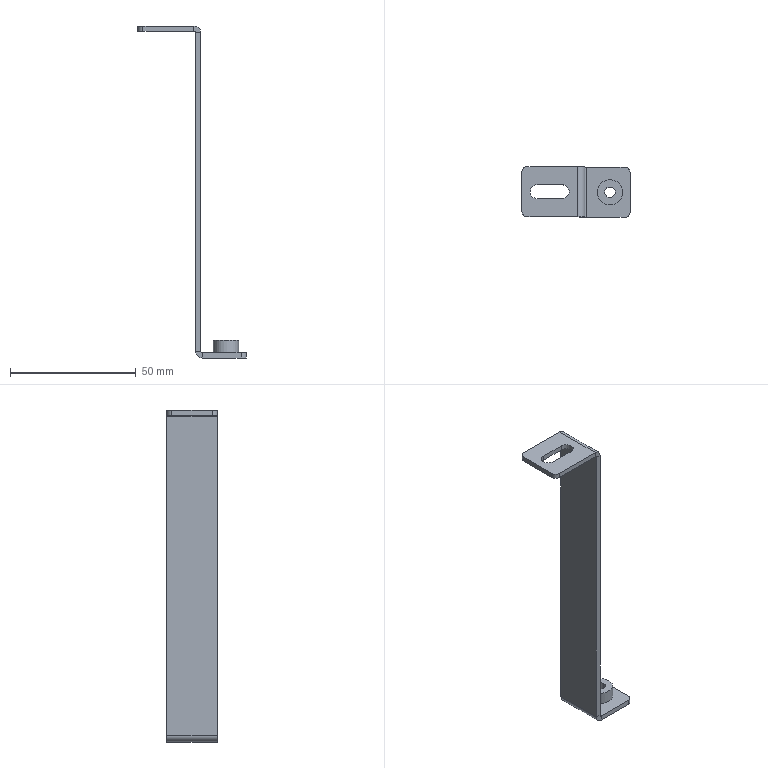Part | STEP file | H_ND24021-01-JG-096-TL | 1 solid | 36 faces | box 43 x 20 x 132 mm | volume 6992 mm3 | plane 21 | cylinder 15 | commonest cylinder face diameters 4 x4 5.5 x3 1.473 x2 4.2 x2 5.473 x2 10 x2